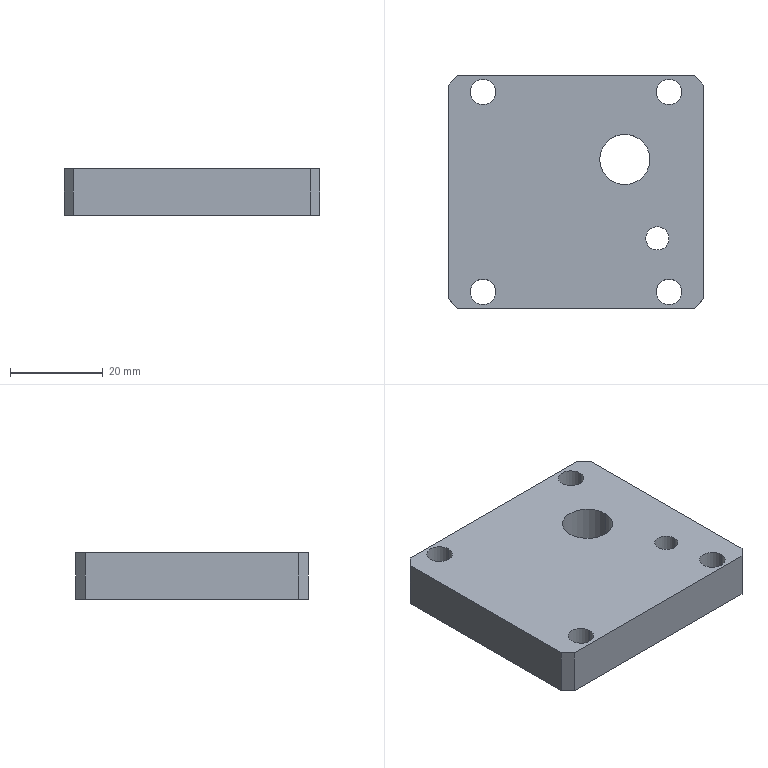Part | STEP file | GLSJ-10-06 | 1 solid | 22 faces | box 55 x 50 x 10 mm | volume 25357 mm3 | cylinder 12 | plane 10 | commonest cylinder face diameters 5.5 x8 5 x2 10.8 x2